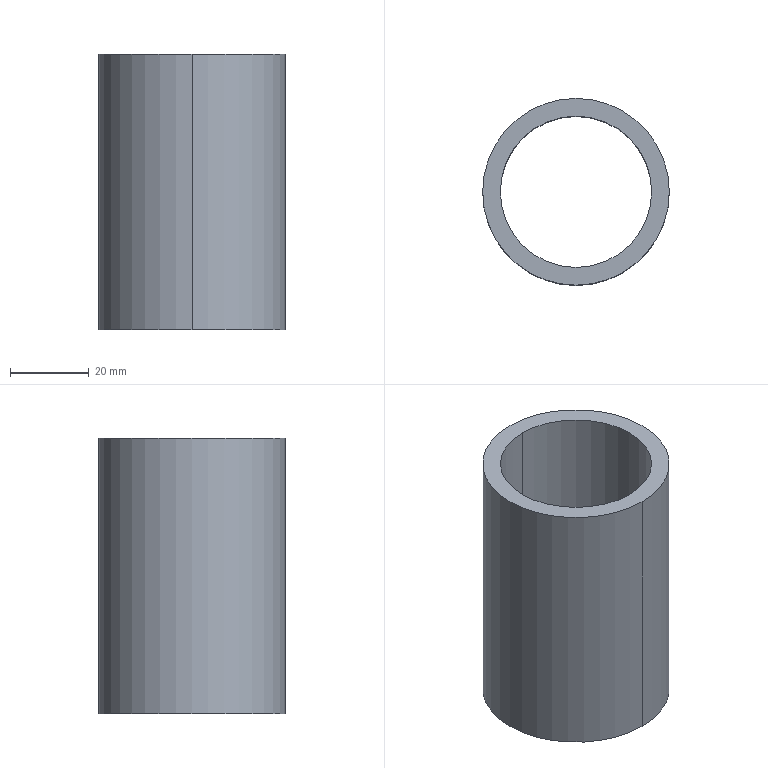Part | NX | features MYKP38-200_3 2 | 1 solid | 6 faces | box 47.5 x 47.5 x 70 mm | volume 42553 mm3 | cylinder 4 | plane 2 | commonest cylinder face diameters 38.5 x2 47.5 x2
STEP:
#1=CARTESIAN_POINT('',(1759.977,-288.655,-110.001));
#2=VERTEX_POINT('',#1);
#3=CARTESIAN_POINT('',(1759.977,-336.155,-110.001));
#4=VERTEX_POINT('',#3);
#5=CARTESIAN_POINT('',(1759.977,-312.405,-110.001));
#6=DIRECTION('',(0.,0.,-1.));
#7=DIRECTION('',(0.,1.,0.));
#8=AXIS2_PLACEMENT_3D('',#5,#6,#7);
#9=CIRCLE('',#8,23.75);
#10=EDGE_CURVE('',#2,#4,#9,.T.);
#11=ORIENTED_EDGE('',*,*,#10,.F.);
#12=CARTESIAN_POINT('',(1759.977,-312.405,-110.001));
#13=DIRECTION('',(0.,0.,-1.));
#14=DIRECTION('',(0.,-1.,0.));
#15=AXIS2_PLACEMENT_3D('',#12,#13,#14);
#16=CIRCLE('',#15,23.75);
#17=EDGE_CURVE('',#4,#2,#16,.T.);
#18=ORIENTED_EDGE('',*,*,#17,.F.);
#19=EDGE_LOOP('',(#11,#18));
#20=FACE_BOUND('',#19,.T.);
#21=CARTESIAN_POINT('',(1759.977,-293.155,-110.001));
#22=VERTEX_POINT('',#21);
#23=CARTESIAN_POINT('',(1759.977,-331.655,-110.001));
#24=VERTEX_POINT('',#23);
#25=CARTESIAN_POINT('',(1759.977,-312.405,-110.001));
#26=DIRECTION('',(0.,0.,1.));
#27=DIRECTION('',(0.,1.,0.));
#28=AXIS2_PLACEMENT_3D('',#25,#26,#27);
#29=CIRCLE('',#28,19.25);
#30=EDGE_CURVE('',#22,#24,#29,.T.);
#31=ORIENTED_EDGE('',*,*,#30,.F.);
#32=CARTESIAN_POINT('',(1759.977,-312.405,-110.001));
#33=DIRECTION('',(0.,0.,1.));
#34=DIRECTION('',(0.,-1.,0.));
#35=AXIS2_PLACEMENT_3D('',#32,#33,#34);
#36=CIRCLE('',#35,19.25);
#37=EDGE_CURVE('',#24,#22,#36,.T.);
#38=ORIENTED_EDGE('',*,*,#37,.F.);
#39=EDGE_LOOP('',(#31,#38));
#40=FACE_BOUND('',#39,.T.);
#41=CARTESIAN_POINT('',(1736.227,-312.405,-110.001));
#42=DIRECTION('',(0.,0.,1.));
#43=DIRECTION('',(0.,-1.,0.));
#44=AXIS2_PLACEMENT_3D('',#41,#42,#43);
#45=PLANE('',#44);
#46=ADVANCED_FACE('',(#20,#40),#45,.T.);
#47=CARTESIAN_POINT('',(1759.977,-288.655,-180.001));
#48=VERTEX_POINT('',#47);
#49=CARTESIAN_POINT('',(1759.977,-336.155,-180.001));
#50=VERTEX_POINT('',#49);
#51=CARTESIAN_POINT('',(1759.977,-312.405,-180.001));
#52=DIRECTION('',(0.,0.,1.));
#53=DIRECTION('',(0.,1.,0.));
#54=AXIS2_PLACEMENT_3D('',#51,#52,#53);
#55=CIRCLE('',#54,23.75);
#56=EDGE_CURVE('',#48,#50,#55,.T.);
#57=ORIENTED_EDGE('',*,*,#56,.T.);
#58=CARTESIAN_POINT('',(1759.977,-336.155,-110.001));
#59=DIRECTION('',(0.,0.,-1.));
#60=VECTOR('',#59,1000.);
#61=LINE('',#58,#60);
#62=EDGE_CURVE('',#50,#4,#61,.F.);
#63=ORIENTED_EDGE('',*,*,#62,.T.);
#64=ORIENTED_EDGE('',*,*,#17,.T.);
#65=CARTESIAN_POINT('',(1759.977,-288.655,-110.001));
#66=DIRECTION('',(0.,0.,-1.));
#67=VECTOR('',#66,1000.);
#68=LINE('',#65,#67);
#69=EDGE_CURVE('',#2,#48,#68,.T.);
#70=ORIENTED_EDGE('',*,*,#69,.T.);
#71=EDGE_LOOP('',(#57,#63,#64,#70));
#72=FACE_BOUND('',#71,.T.);
#73=CARTESIAN_POINT('',(1759.977,-312.405,-20.001));
#74=DIRECTION('',(0.,0.,-1.));
#75=DIRECTION('',(-1.,0.,0.));
#76=AXIS2_PLACEMENT_3D('',#73,#74,#75);
#77=CYLINDRICAL_SURFACE('',#76,23.75);
#78=ADVANCED_FACE('',(#72),#77,.T.);
#79=CARTESIAN_POINT('',(1783.727,-312.405,-180.001));
#80=VERTEX_POINT('',#79);
#81=CARTESIAN_POINT('',(1759.977,-312.405,-180.001));
#82=DIRECTION('',(0.,0.,1.));
#83=DIRECTION('',(1.,0.,0.));
#84=AXIS2_PLACEMENT_3D('',#81,#82,#83);
#85=CIRCLE('',#84,23.75);
#86=EDGE_CURVE('',#80,#48,#85,.T.);
#87=ORIENTED_EDGE('',*,*,#86,.F.);
#88=CARTESIAN_POINT('',(1759.977,-312.405,-180.001));
#89=DIRECTION('',(0.,0.,1.));
#90=DIRECTION('',(0.,-1.,0.));
#91=AXIS2_PLACEMENT_3D('',#88,#89,#90);
#92=CIRCLE('',#91,23.75);
#93=EDGE_CURVE('',#50,#80,#92,.T.);
#94=ORIENTED_EDGE('',*,*,#93,.F.);
#95=ORIENTED_EDGE('',*,*,#56,.F.);
#96=EDGE_LOOP('',(#87,#94,#95));
#97=FACE_BOUND('',#96,.T.);
#98=CARTESIAN_POINT('',(1740.727,-312.405,-180.001));
#99=VERTEX_POINT('',#98);
#100=CARTESIAN_POINT('',(1759.977,-293.155,-180.001));
#101=VERTEX_POINT('',#100);
#102=CARTESIAN_POINT('',(1759.977,-312.405,-180.001));
#103=DIRECTION('',(0.,0.,-1.));
#104=DIRECTION('',(-1.,0.,0.));
#105=AXIS2_PLACEMENT_3D('',#102,#103,#104);
#106=CIRCLE('',#105,19.25);
#107=EDGE_CURVE('',#99,#101,#106,.T.);
#108=ORIENTED_EDGE('',*,*,#107,.F.);
#109=CARTESIAN_POINT('',(1759.977,-331.655,-180.001));
#110=VERTEX_POINT('',#109);
#111=CARTESIAN_POINT('',(1759.977,-312.405,-180.001));
#112=DIRECTION('',(0.,0.,-1.));
#113=DIRECTION('',(0.,-1.,0.));
#114=AXIS2_PLACEMENT_3D('',#111,#112,#113);
#115=CIRCLE('',#114,19.25);
#116=EDGE_CURVE('',#110,#99,#115,.T.);
#117=ORIENTED_EDGE('',*,*,#116,.F.);
#118=CARTESIAN_POINT('',(1779.227,-312.405,-180.001));
#119=VERTEX_POINT('',#118);
#120=CARTESIAN_POINT('',(1759.977,-312.405,-180.001));
#121=DIRECTION('',(0.,0.,-1.));
#122=DIRECTION('',(1.,0.,0.));
#123=AXIS2_PLACEMENT_3D('',#120,#121,#122);
#124=CIRCLE('',#123,19.25);
#125=EDGE_CURVE('',#119,#110,#124,.T.);
#126=ORIENTED_EDGE('',*,*,#125,.F.);
#127=CARTESIAN_POINT('',(1759.977,-312.405,-180.001));
#128=DIRECTION('',(0.,0.,-1.));
#129=DIRECTION('',(0.,1.,0.));
#130=AXIS2_PLACEMENT_3D('',#127,#128,#129);
#131=CIRCLE('',#130,19.25);
#132=EDGE_CURVE('',#101,#119,#131,.T.);
#133=ORIENTED_EDGE('',*,*,#132,.F.);
#134=EDGE_LOOP('',(#108,#117,#126,#133));
#135=FACE_BOUND('',#134,.T.);
#136=CARTESIAN_POINT('',(1759.977,-312.405,-180.001));
#137=DIRECTION('',(0.,0.,1.));
#138=DIRECTION('',(0.,-1.,0.));
#139=AXIS2_PLACEMENT_3D('',#136,#137,#138);
#140=PLANE('',#139);
#141=ADVANCED_FACE('',(#97,#135),#140,.F.);
#142=ORIENTED_EDGE('',*,*,#93,.T.);
#143=ORIENTED_EDGE('',*,*,#86,.T.);
#144=ORIENTED_EDGE('',*,*,#69,.F.);
#145=ORIENTED_EDGE('',*,*,#10,.T.);
#146=ORIENTED_EDGE('',*,*,#62,.F.);
#147=EDGE_LOOP('',(#142,#143,#144,#145,#146));
#148=FACE_BOUND('',#147,.T.);
#149=CARTESIAN_POINT('',(1759.977,-312.405,-20.001));
#150=DIRECTION('',(0.,0.,-1.));
#151=DIRECTION('',(-1.,0.,0.));
#152=AXIS2_PLACEMENT_3D('',#149,#150,#151);
#153=CYLINDRICAL_SURFACE('',#152,23.75);
#154=ADVANCED_FACE('',(#148),#153,.T.);
#155=ORIENTED_EDGE('',*,*,#116,.T.);
#156=ORIENTED_EDGE('',*,*,#107,.T.);
#157=CARTESIAN_POINT('',(1759.977,-293.155,-110.001));
#158=DIRECTION('',(0.,0.,-1.));
#159=VECTOR('',#158,1000.);
#160=LINE('',#157,#159);
#161=EDGE_CURVE('',#101,#22,#160,.F.);
#162=ORIENTED_EDGE('',*,*,#161,.T.);
#163=ORIENTED_EDGE('',*,*,#30,.T.);
#164=CARTESIAN_POINT('',(1759.977,-331.655,-110.001));
#165=DIRECTION('',(0.,0.,-1.));
#166=VECTOR('',#165,1000.);
#167=LINE('',#164,#166);
#168=EDGE_CURVE('',#24,#110,#167,.T.);
#169=ORIENTED_EDGE('',*,*,#168,.T.);
#170=EDGE_LOOP('',(#155,#156,#162,#163,#169));
#171=FACE_BOUND('',#170,.T.);
#172=CARTESIAN_POINT('',(1759.977,-312.405,-20.001));
#173=DIRECTION('',(0.,0.,-1.));
#174=DIRECTION('',(-1.,0.,0.));
#175=AXIS2_PLACEMENT_3D('',#172,#173,#174);
#176=CYLINDRICAL_SURFACE('',#175,19.25);
#177=ADVANCED_FACE('',(#171),#176,.F.);
#178=ORIENTED_EDGE('',*,*,#132,.T.);
#179=ORIENTED_EDGE('',*,*,#125,.T.);
#180=ORIENTED_EDGE('',*,*,#168,.F.);
#181=ORIENTED_EDGE('',*,*,#37,.T.);
#182=ORIENTED_EDGE('',*,*,#161,.F.);
#183=EDGE_LOOP('',(#178,#179,#180,#181,#182));
#184=FACE_BOUND('',#183,.T.);
#185=CARTESIAN_POINT('',(1759.977,-312.405,-20.001));
#186=DIRECTION('',(0.,0.,-1.));
#187=DIRECTION('',(-1.,0.,0.));
#188=AXIS2_PLACEMENT_3D('',#185,#186,#187);
#189=CYLINDRICAL_SURFACE('',#188,19.25);
#190=ADVANCED_FACE('',(#184),#189,.F.);
#191=CLOSED_SHELL('',(#46,#78,#141,#154,#177,#190));
#192=MANIFOLD_SOLID_BREP('',#191);
#193=(LENGTH_UNIT()NAMED_UNIT(*)SI_UNIT(.MILLI.,.METRE.));
#194=UNCERTAINTY_MEASURE_WITH_UNIT(LENGTH_MEASURE(0.00001),#193,'','');
#195=(NAMED_UNIT(*)PLANE_ANGLE_UNIT()SI_UNIT($,.RADIAN.));
#196=(NAMED_UNIT(*)SI_UNIT($,.STERADIAN.)SOLID_ANGLE_UNIT());
#197=(GEOMETRIC_REPRESENTATION_CONTEXT(3)GLOBAL_UNCERTAINTY_ASSIGNED_CONTEXT((#194))GLOBAL_UNIT_ASSIGNED_CONTEXT((#193,#195,#196))REPRESENTATION_CONTEXT('',''));
#198=ADVANCED_BREP_SHAPE_REPRESENTATION('',(#192),#197);